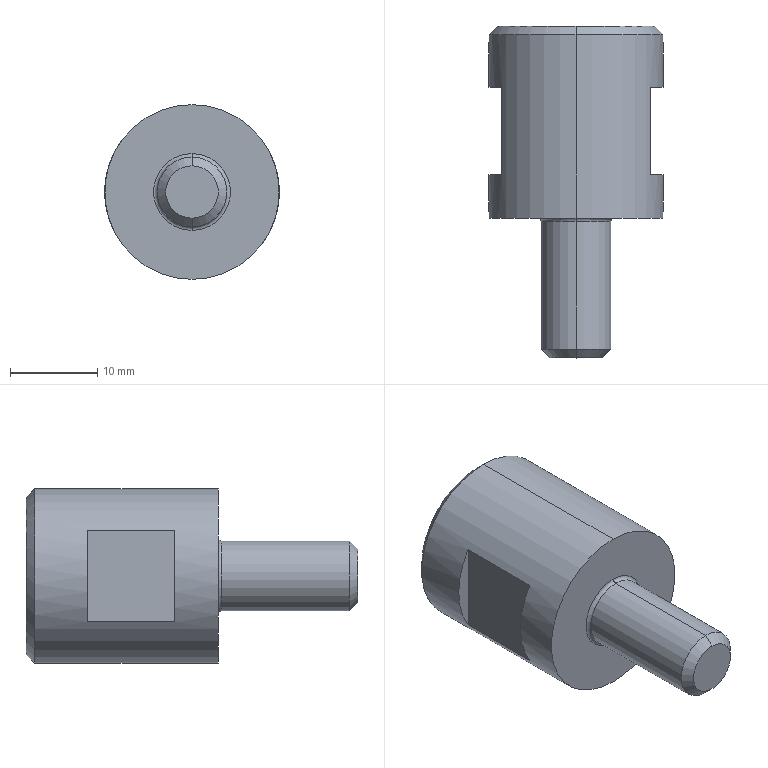Part | STEP file | OP10-125_seal rod dia7 | 1 solid | 35 faces | box 20 x 38 x 20 mm | volume 6478 mm3 | plane 13 | cylinder 12 | cone 8 | torus 2 | commonest cylinder face diameters 4 x4 8 x2 12.245 x2 14.5 x2 20 x2